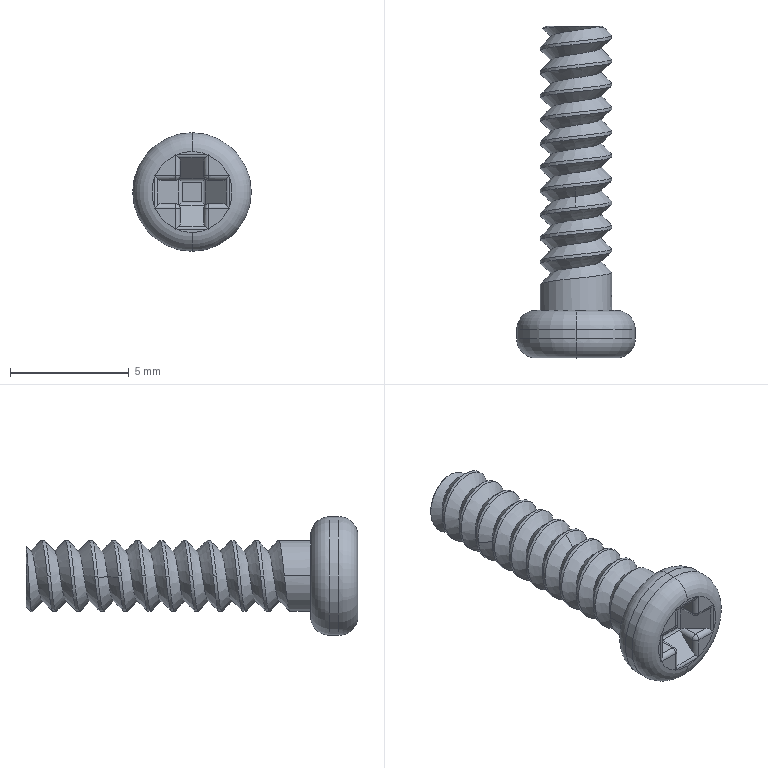Part | STEP file | LUODING_5_1 | 1 solid | 85 faces | box 5 x 14 x 5 mm | volume 98.522 mm3 | cylinder 44 | plane 25 | spline 7 | torus 4 | sphere 4 | cone 1 | commonest cylinder face diameters 3 x22 0.4 x20 5 x2